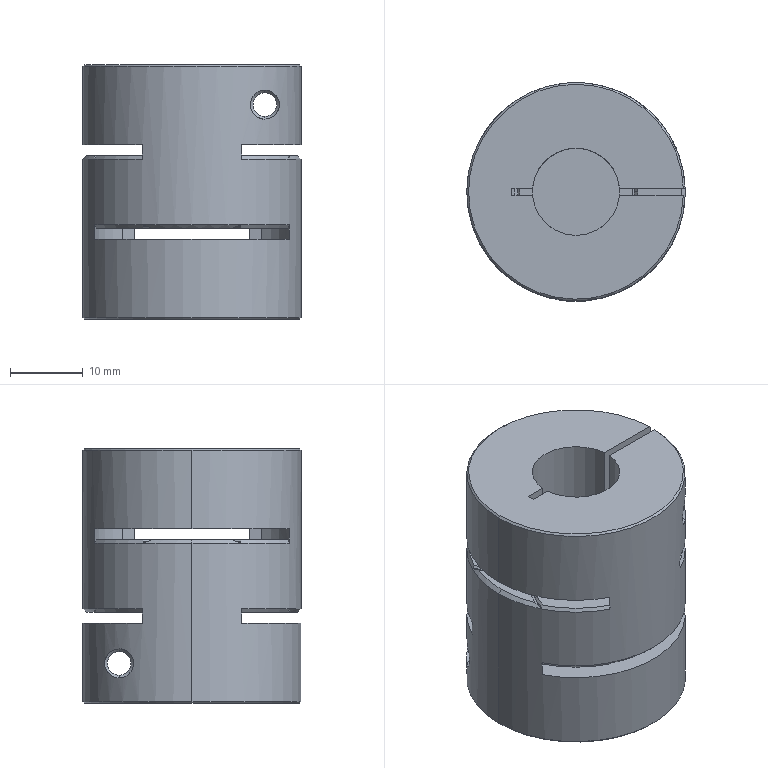Part | SolidWorks | features BaseBody 1 | 1 solid | 181 faces | box 30 x 30 x 35 mm | volume 19054 mm3 | cone 65 | plane 64 | cylinder 52 | commonest cylinder face diameters 16.982 x16 16 x10 4 x8 12 x6 3.242 x4 7.5 x4